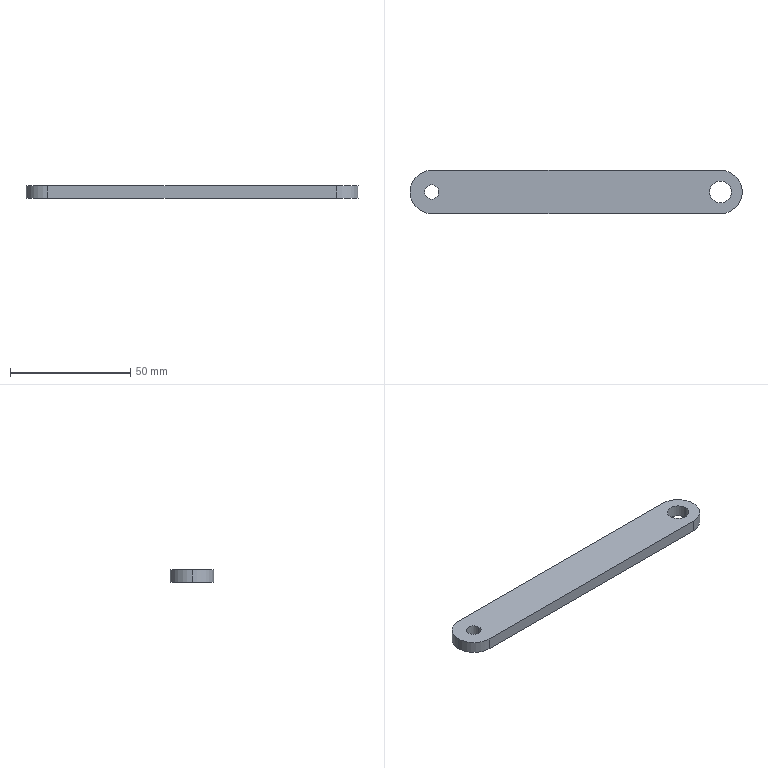Part | SolidWorks | features ICE 2, Extrusion 1 | 1 solid | 11 faces | box 138 x 18 x 5 mm | volume 11613 mm3 | cylinder 7 | plane 4 | commonest cylinder face diameters 18 x3 6 x2 9 x2
STEP:
#1=CARTESIAN_POINT('',(124.5,0.,0.));
#2=VERTEX_POINT('',#1);
#3=CARTESIAN_POINT('',(115.5,0.,0.));
#4=VERTEX_POINT('',#3);
#5=CARTESIAN_POINT('',(120.,0.,0.));
#6=DIRECTION('',(0.,0.,-1.));
#7=DIRECTION('',(1.,0.,0.));
#8=AXIS2_PLACEMENT_3D('',#5,#6,#7);
#9=CIRCLE('',#8,4.5);
#10=EDGE_CURVE('',#2,#4,#9,.T.);
#11=ORIENTED_EDGE('',*,*,#10,.T.);
#12=CARTESIAN_POINT('',(115.5,0.,5.));
#13=VERTEX_POINT('',#12);
#14=CARTESIAN_POINT('',(115.5,0.,-25.456));
#15=DIRECTION('',(0.,0.,1.));
#16=VECTOR('',#15,1000.);
#17=LINE('',#14,#16);
#18=EDGE_CURVE('',#4,#13,#17,.T.);
#19=ORIENTED_EDGE('',*,*,#18,.T.);
#20=CARTESIAN_POINT('',(124.5,0.,5.));
#21=VERTEX_POINT('',#20);
#22=CARTESIAN_POINT('',(120.,0.,5.));
#23=DIRECTION('',(0.,0.,1.));
#24=DIRECTION('',(1.,0.,0.));
#25=AXIS2_PLACEMENT_3D('',#22,#23,#24);
#26=CIRCLE('',#25,4.5);
#27=EDGE_CURVE('',#13,#21,#26,.T.);
#28=ORIENTED_EDGE('',*,*,#27,.T.);
#29=CARTESIAN_POINT('',(124.5,0.,-25.456));
#30=DIRECTION('',(0.,0.,1.));
#31=VECTOR('',#30,1000.);
#32=LINE('',#29,#31);
#33=EDGE_CURVE('',#2,#21,#32,.T.);
#34=ORIENTED_EDGE('',*,*,#33,.F.);
#35=EDGE_LOOP('',(#11,#19,#28,#34));
#36=FACE_OUTER_BOUND('',#35,.T.);
#37=CARTESIAN_POINT('',(120.,0.,-25.456));
#38=DIRECTION('',(0.,0.,1.));
#39=DIRECTION('',(1.,0.,0.));
#40=AXIS2_PLACEMENT_3D('',#37,#38,#39);
#41=CYLINDRICAL_SURFACE('',#40,4.5);
#42=ADVANCED_FACE('',(#36),#41,.F.);
#43=CARTESIAN_POINT('',(-3.,0.,5.));
#44=VERTEX_POINT('',#43);
#45=CARTESIAN_POINT('',(3.,0.,5.));
#46=VERTEX_POINT('',#45);
#47=CARTESIAN_POINT('',(0.,0.,5.));
#48=DIRECTION('',(0.,0.,1.));
#49=DIRECTION('',(1.,0.,0.));
#50=AXIS2_PLACEMENT_3D('',#47,#48,#49);
#51=CIRCLE('',#50,3.);
#52=EDGE_CURVE('',#44,#46,#51,.T.);
#53=ORIENTED_EDGE('',*,*,#52,.T.);
#54=CARTESIAN_POINT('',(3.,0.,0.));
#55=VERTEX_POINT('',#54);
#56=CARTESIAN_POINT('',(3.,0.,5.));
#57=DIRECTION('',(0.,0.,-1.));
#58=VECTOR('',#57,1000.);
#59=LINE('',#56,#58);
#60=EDGE_CURVE('',#46,#55,#59,.T.);
#61=ORIENTED_EDGE('',*,*,#60,.T.);
#62=CARTESIAN_POINT('',(-3.,0.,0.));
#63=VERTEX_POINT('',#62);
#64=CARTESIAN_POINT('',(0.,0.,0.));
#65=DIRECTION('',(0.,0.,1.));
#66=DIRECTION('',(1.,0.,0.));
#67=AXIS2_PLACEMENT_3D('',#64,#65,#66);
#68=CIRCLE('',#67,3.);
#69=EDGE_CURVE('',#63,#55,#68,.T.);
#70=ORIENTED_EDGE('',*,*,#69,.F.);
#71=CARTESIAN_POINT('',(-3.,0.,5.));
#72=DIRECTION('',(0.,0.,-1.));
#73=VECTOR('',#72,1000.);
#74=LINE('',#71,#73);
#75=EDGE_CURVE('',#44,#63,#74,.T.);
#76=ORIENTED_EDGE('',*,*,#75,.F.);
#77=EDGE_LOOP('',(#53,#61,#70,#76));
#78=FACE_OUTER_BOUND('',#77,.T.);
#79=CARTESIAN_POINT('',(0.,0.,5.));
#80=DIRECTION('',(0.,0.,-1.));
#81=DIRECTION('',(-1.,0.,0.));
#82=AXIS2_PLACEMENT_3D('',#79,#80,#81);
#83=CYLINDRICAL_SURFACE('',#82,3.);
#84=ADVANCED_FACE('',(#78),#83,.F.);
#85=CARTESIAN_POINT('',(-9.,0.,5.));
#86=VERTEX_POINT('',#85);
#87=CARTESIAN_POINT('',(0.,-9.,5.));
#88=VERTEX_POINT('',#87);
#89=CARTESIAN_POINT('',(0.,0.,5.));
#90=DIRECTION('',(0.,0.,1.));
#91=DIRECTION('',(1.,0.,0.));
#92=AXIS2_PLACEMENT_3D('',#89,#90,#91);
#93=CIRCLE('',#92,9.);
#94=EDGE_CURVE('',#86,#88,#93,.T.);
#95=ORIENTED_EDGE('',*,*,#94,.F.);
#96=CARTESIAN_POINT('',(-9.,0.,0.));
#97=VERTEX_POINT('',#96);
#98=CARTESIAN_POINT('',(-9.,0.,5.));
#99=DIRECTION('',(0.,0.,-1.));
#100=VECTOR('',#99,1000.);
#101=LINE('',#98,#100);
#102=EDGE_CURVE('',#86,#97,#101,.T.);
#103=ORIENTED_EDGE('',*,*,#102,.T.);
#104=CARTESIAN_POINT('',(0.,-9.,0.));
#105=VERTEX_POINT('',#104);
#106=CARTESIAN_POINT('',(0.,0.,0.));
#107=DIRECTION('',(0.,0.,1.));
#108=DIRECTION('',(1.,0.,0.));
#109=AXIS2_PLACEMENT_3D('',#106,#107,#108);
#110=CIRCLE('',#109,9.);
#111=EDGE_CURVE('',#97,#105,#110,.T.);
#112=ORIENTED_EDGE('',*,*,#111,.T.);
#113=CARTESIAN_POINT('',(0.,-9.,5.));
#114=DIRECTION('',(0.,0.,-1.));
#115=VECTOR('',#114,1000.);
#116=LINE('',#113,#115);
#117=EDGE_CURVE('',#88,#105,#116,.T.);
#118=ORIENTED_EDGE('',*,*,#117,.F.);
#119=EDGE_LOOP('',(#95,#103,#112,#118));
#120=FACE_OUTER_BOUND('',#119,.T.);
#121=CARTESIAN_POINT('',(0.,0.,5.));
#122=DIRECTION('',(0.,0.,-1.));
#123=DIRECTION('',(-1.,0.,0.));
#124=AXIS2_PLACEMENT_3D('',#121,#122,#123);
#125=CYLINDRICAL_SURFACE('',#124,9.);
#126=ADVANCED_FACE('',(#120),#125,.T.);
#127=CARTESIAN_POINT('',(120.,-9.,5.));
#128=VERTEX_POINT('',#127);
#129=CARTESIAN_POINT('',(0.,-9.,5.));
#130=DIRECTION('',(1.,0.,0.));
#131=VECTOR('',#130,1000.);
#132=LINE('',#129,#131);
#133=EDGE_CURVE('',#88,#128,#132,.T.);
#134=ORIENTED_EDGE('',*,*,#133,.T.);
#135=CARTESIAN_POINT('',(120.,9.,5.));
#136=VERTEX_POINT('',#135);
#137=CARTESIAN_POINT('',(120.,0.,5.));
#138=DIRECTION('',(0.,0.,1.));
#139=DIRECTION('',(1.,0.,0.));
#140=AXIS2_PLACEMENT_3D('',#137,#138,#139);
#141=CIRCLE('',#140,9.);
#142=EDGE_CURVE('',#128,#136,#141,.T.);
#143=ORIENTED_EDGE('',*,*,#142,.T.);
#144=CARTESIAN_POINT('',(0.,9.,5.));
#145=VERTEX_POINT('',#144);
#146=CARTESIAN_POINT('',(0.,9.,5.));
#147=DIRECTION('',(-1.,0.,0.));
#148=VECTOR('',#147,1000.);
#149=LINE('',#146,#148);
#150=EDGE_CURVE('',#136,#145,#149,.T.);
#151=ORIENTED_EDGE('',*,*,#150,.T.);
#152=CARTESIAN_POINT('',(0.,0.,5.));
#153=DIRECTION('',(0.,0.,1.));
#154=DIRECTION('',(1.,0.,0.));
#155=AXIS2_PLACEMENT_3D('',#152,#153,#154);
#156=CIRCLE('',#155,9.);
#157=EDGE_CURVE('',#145,#86,#156,.T.);
#158=ORIENTED_EDGE('',*,*,#157,.T.);
#159=ORIENTED_EDGE('',*,*,#94,.T.);
#160=EDGE_LOOP('',(#134,#143,#151,#158,#159));
#161=FACE_OUTER_BOUND('',#160,.T.);
#162=ORIENTED_EDGE('',*,*,#52,.F.);
#163=CARTESIAN_POINT('',(0.,0.,5.));
#164=DIRECTION('',(0.,0.,1.));
#165=DIRECTION('',(1.,0.,0.));
#166=AXIS2_PLACEMENT_3D('',#163,#164,#165);
#167=CIRCLE('',#166,3.);
#168=EDGE_CURVE('',#46,#44,#167,.T.);
#169=ORIENTED_EDGE('',*,*,#168,.F.);
#170=EDGE_LOOP('',(#162,#169));
#171=FACE_BOUND('',#170,.T.);
#172=CARTESIAN_POINT('',(120.,0.,5.));
#173=DIRECTION('',(0.,0.,1.));
#174=DIRECTION('',(1.,0.,0.));
#175=AXIS2_PLACEMENT_3D('',#172,#173,#174);
#176=CIRCLE('',#175,4.5);
#177=EDGE_CURVE('',#21,#13,#176,.T.);
#178=ORIENTED_EDGE('',*,*,#177,.F.);
#179=ORIENTED_EDGE('',*,*,#27,.F.);
#180=EDGE_LOOP('',(#178,#179));
#181=FACE_BOUND('',#180,.T.);
#182=CARTESIAN_POINT('',(0.,0.,5.));
#183=DIRECTION('',(0.,0.,1.));
#184=DIRECTION('',(1.,0.,0.));
#185=AXIS2_PLACEMENT_3D('',#182,#183,#184);
#186=PLANE('',#185);
#187=ADVANCED_FACE('',(#161,#171,#181),#186,.T.);
#188=CARTESIAN_POINT('',(120.,9.,0.));
#189=VERTEX_POINT('',#188);
#190=CARTESIAN_POINT('',(0.,9.,0.));
#191=VERTEX_POINT('',#190);
#192=CARTESIAN_POINT('',(0.,9.,0.));
#193=DIRECTION('',(-1.,0.,0.));
#194=VECTOR('',#193,1000.);
#195=LINE('',#192,#194);
#196=EDGE_CURVE('',#189,#191,#195,.T.);
#197=ORIENTED_EDGE('',*,*,#196,.F.);
#198=CARTESIAN_POINT('',(120.,-9.,0.));
#199=VERTEX_POINT('',#198);
#200=CARTESIAN_POINT('',(120.,0.,0.));
#201=DIRECTION('',(0.,0.,1.));
#202=DIRECTION('',(1.,0.,0.));
#203=AXIS2_PLACEMENT_3D('',#200,#201,#202);
#204=CIRCLE('',#203,9.);
#205=EDGE_CURVE('',#199,#189,#204,.T.);
#206=ORIENTED_EDGE('',*,*,#205,.F.);
#207=CARTESIAN_POINT('',(0.,-9.,0.));
#208=DIRECTION('',(1.,0.,0.));
#209=VECTOR('',#208,1000.);
#210=LINE('',#207,#209);
#211=EDGE_CURVE('',#105,#199,#210,.T.);
#212=ORIENTED_EDGE('',*,*,#211,.F.);
#213=ORIENTED_EDGE('',*,*,#111,.F.);
#214=CARTESIAN_POINT('',(0.,0.,0.));
#215=DIRECTION('',(0.,0.,1.));
#216=DIRECTION('',(1.,0.,0.));
#217=AXIS2_PLACEMENT_3D('',#214,#215,#216);
#218=CIRCLE('',#217,9.);
#219=EDGE_CURVE('',#191,#97,#218,.T.);
#220=ORIENTED_EDGE('',*,*,#219,.F.);
#221=EDGE_LOOP('',(#197,#206,#212,#213,#220));
#222=FACE_OUTER_BOUND('',#221,.T.);
#223=ORIENTED_EDGE('',*,*,#69,.T.);
#224=CARTESIAN_POINT('',(0.,0.,0.));
#225=DIRECTION('',(0.,0.,1.));
#226=DIRECTION('',(1.,0.,0.));
#227=AXIS2_PLACEMENT_3D('',#224,#225,#226);
#228=CIRCLE('',#227,3.);
#229=EDGE_CURVE('',#55,#63,#228,.T.);
#230=ORIENTED_EDGE('',*,*,#229,.T.);
#231=EDGE_LOOP('',(#223,#230));
#232=FACE_BOUND('',#231,.T.);
#233=ORIENTED_EDGE('',*,*,#10,.F.);
#234=CARTESIAN_POINT('',(120.,0.,0.));
#235=DIRECTION('',(0.,0.,-1.));
#236=DIRECTION('',(1.,0.,0.));
#237=AXIS2_PLACEMENT_3D('',#234,#235,#236);
#238=CIRCLE('',#237,4.5);
#239=EDGE_CURVE('',#4,#2,#238,.T.);
#240=ORIENTED_EDGE('',*,*,#239,.F.);
#241=EDGE_LOOP('',(#233,#240));
#242=FACE_BOUND('',#241,.T.);
#243=CARTESIAN_POINT('',(0.,0.,0.));
#244=DIRECTION('',(0.,0.,1.));
#245=DIRECTION('',(1.,0.,0.));
#246=AXIS2_PLACEMENT_3D('',#243,#244,#245);
#247=PLANE('',#246);
#248=ADVANCED_FACE('',(#222,#232,#242),#247,.F.);
#249=ORIENTED_EDGE('',*,*,#102,.F.);
#250=ORIENTED_EDGE('',*,*,#157,.F.);
#251=CARTESIAN_POINT('',(0.,9.,5.));
#252=DIRECTION('',(0.,0.,-1.));
#253=VECTOR('',#252,1000.);
#254=LINE('',#251,#253);
#255=EDGE_CURVE('',#145,#191,#254,.T.);
#256=ORIENTED_EDGE('',*,*,#255,.T.);
#257=ORIENTED_EDGE('',*,*,#219,.T.);
#258=EDGE_LOOP('',(#249,#250,#256,#257));
#259=FACE_OUTER_BOUND('',#258,.T.);
#260=CARTESIAN_POINT('',(0.,0.,5.));
#261=DIRECTION('',(0.,0.,-1.));
#262=DIRECTION('',(-1.,0.,0.));
#263=AXIS2_PLACEMENT_3D('',#260,#261,#262);
#264=CYLINDRICAL_SURFACE('',#263,9.);
#265=ADVANCED_FACE('',(#259),#264,.T.);
#266=ORIENTED_EDGE('',*,*,#211,.T.);
#267=CARTESIAN_POINT('',(120.,-9.,5.));
#268=DIRECTION('',(0.,0.,-1.));
#269=VECTOR('',#268,1000.);
#270=LINE('',#267,#269);
#271=EDGE_CURVE('',#128,#199,#270,.T.);
#272=ORIENTED_EDGE('',*,*,#271,.F.);
#273=ORIENTED_EDGE('',*,*,#133,.F.);
#274=ORIENTED_EDGE('',*,*,#117,.T.);
#275=EDGE_LOOP('',(#266,#272,#273,#274));
#276=FACE_OUTER_BOUND('',#275,.T.);
#277=CARTESIAN_POINT('',(0.,-9.,5.));
#278=DIRECTION('',(0.,1.,0.));
#279=DIRECTION('',(0.,0.,1.));
#280=AXIS2_PLACEMENT_3D('',#277,#278,#279);
#281=PLANE('',#280);
#282=ADVANCED_FACE('',(#276),#281,.F.);
#283=ORIENTED_EDGE('',*,*,#205,.T.);
#284=CARTESIAN_POINT('',(120.,9.,5.));
#285=DIRECTION('',(0.,0.,-1.));
#286=VECTOR('',#285,1000.);
#287=LINE('',#284,#286);
#288=EDGE_CURVE('',#136,#189,#287,.T.);
#289=ORIENTED_EDGE('',*,*,#288,.F.);
#290=ORIENTED_EDGE('',*,*,#142,.F.);
#291=ORIENTED_EDGE('',*,*,#271,.T.);
#292=EDGE_LOOP('',(#283,#289,#290,#291));
#293=FACE_OUTER_BOUND('',#292,.T.);
#294=CARTESIAN_POINT('',(120.,0.,5.));
#295=DIRECTION('',(0.,0.,-1.));
#296=DIRECTION('',(-1.,0.,0.));
#297=AXIS2_PLACEMENT_3D('',#294,#295,#296);
#298=CYLINDRICAL_SURFACE('',#297,9.);
#299=ADVANCED_FACE('',(#293),#298,.T.);
#300=ORIENTED_EDGE('',*,*,#196,.T.);
#301=ORIENTED_EDGE('',*,*,#255,.F.);
#302=ORIENTED_EDGE('',*,*,#150,.F.);
#303=ORIENTED_EDGE('',*,*,#288,.T.);
#304=EDGE_LOOP('',(#300,#301,#302,#303));
#305=FACE_OUTER_BOUND('',#304,.T.);
#306=CARTESIAN_POINT('',(0.,9.,5.));
#307=DIRECTION('',(0.,-1.,0.));
#308=DIRECTION('',(0.,0.,-1.));
#309=AXIS2_PLACEMENT_3D('',#306,#307,#308);
#310=PLANE('',#309);
#311=ADVANCED_FACE('',(#305),#310,.F.);
#312=ORIENTED_EDGE('',*,*,#60,.F.);
#313=ORIENTED_EDGE('',*,*,#168,.T.);
#314=ORIENTED_EDGE('',*,*,#75,.T.);
#315=ORIENTED_EDGE('',*,*,#229,.F.);
#316=EDGE_LOOP('',(#312,#313,#314,#315));
#317=FACE_OUTER_BOUND('',#316,.T.);
#318=CARTESIAN_POINT('',(0.,0.,5.));
#319=DIRECTION('',(0.,0.,-1.));
#320=DIRECTION('',(-1.,0.,0.));
#321=AXIS2_PLACEMENT_3D('',#318,#319,#320);
#322=CYLINDRICAL_SURFACE('',#321,3.);
#323=ADVANCED_FACE('',(#317),#322,.F.);
#324=ORIENTED_EDGE('',*,*,#18,.F.);
#325=ORIENTED_EDGE('',*,*,#239,.T.);
#326=ORIENTED_EDGE('',*,*,#33,.T.);
#327=ORIENTED_EDGE('',*,*,#177,.T.);
#328=EDGE_LOOP('',(#324,#325,#326,#327));
#329=FACE_OUTER_BOUND('',#328,.T.);
#330=CARTESIAN_POINT('',(120.,0.,-25.456));
#331=DIRECTION('',(0.,0.,1.));
#332=DIRECTION('',(1.,0.,0.));
#333=AXIS2_PLACEMENT_3D('',#330,#331,#332);
#334=CYLINDRICAL_SURFACE('',#333,4.5);
#335=ADVANCED_FACE('',(#329),#334,.F.);
#336=CLOSED_SHELL('',(#42,#84,#126,#187,#248,#265,#282,#299,#311,#323,#335));
#337=MANIFOLD_SOLID_BREP('',#336);
#338=CARTESIAN_POINT('',(0.,0.,0.));
#339=DIRECTION('',(0.,0.,1.));
#340=DIRECTION('',(1.,0.,0.));
#341=AXIS2_PLACEMENT_3D('',#338,#339,#340);
#342=(LENGTH_UNIT()NAMED_UNIT(*)SI_UNIT(.MILLI.,.METRE.));
#343=UNCERTAINTY_MEASURE_WITH_UNIT(LENGTH_MEASURE(0.00001),#342,'','');
#344=(NAMED_UNIT(*)PLANE_ANGLE_UNIT()SI_UNIT($,.RADIAN.));
#345=(NAMED_UNIT(*)SI_UNIT($,.STERADIAN.)SOLID_ANGLE_UNIT());
#346=(GEOMETRIC_REPRESENTATION_CONTEXT(3)GLOBAL_UNCERTAINTY_ASSIGNED_CONTEXT((#343))GLOBAL_UNIT_ASSIGNED_CONTEXT((#342,#344,#345))REPRESENTATION_CONTEXT('',''));
#347=ADVANCED_BREP_SHAPE_REPRESENTATION('',(#337,#341),#346);